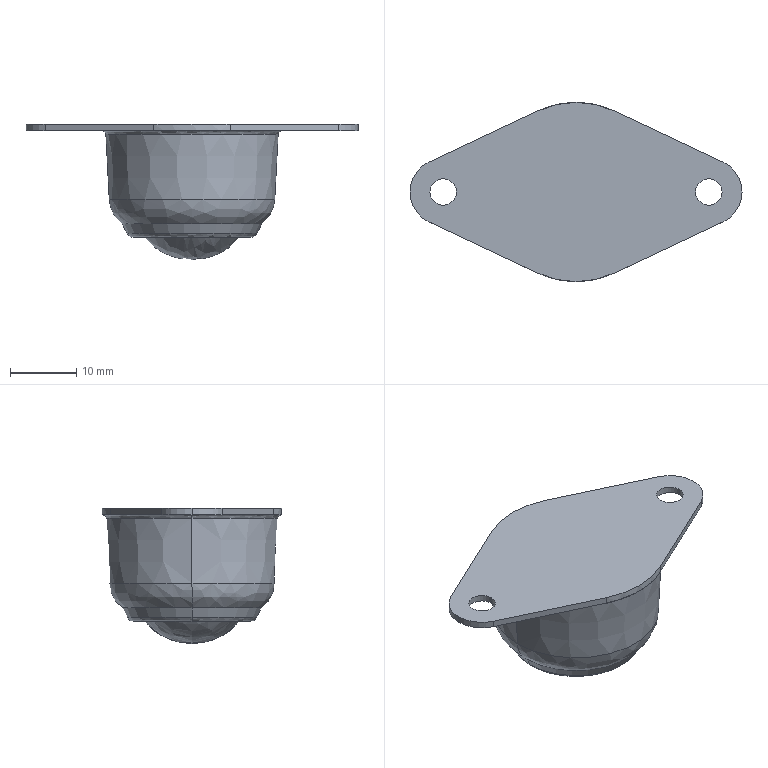Part | SolidWorks | features BaseBody 2 | 2 solids | 32 faces | box 50 x 27 x 20.021 mm | volume 8663 mm3 | cylinder 11 | spline 10 | plane 7 | cone 4 | commonest cylinder face diameters 4 x4 10 x3 15 x2 27 x2
STEP:
#1=CARTESIAN_POINT('',(9.397,0.,-10.));
#2=VERTEX_POINT('',#1);
#3=CARTESIAN_POINT('',(-9.397,0.,-10.));
#4=VERTEX_POINT('',#3);
#5=CARTESIAN_POINT('',(0.,0.,-10.));
#6=DIRECTION('',(0.,0.,-1.));
#7=DIRECTION('',(1.,0.,0.));
#8=AXIS2_PLACEMENT_3D('',#5,#6,#7);
#9=CIRCLE('',#8,9.397);
#10=EDGE_CURVE('',#2,#4,#9,.T.);
#11=ORIENTED_EDGE('',*,*,#10,.F.);
#12=CARTESIAN_POINT('',(0.,0.,-10.));
#13=DIRECTION('',(0.,0.,1.));
#14=DIRECTION('',(1.,0.,0.));
#15=AXIS2_PLACEMENT_3D('',#12,#13,#14);
#16=CIRCLE('',#15,9.397);
#17=EDGE_CURVE('',#2,#4,#16,.T.);
#18=ORIENTED_EDGE('',*,*,#17,.T.);
#19=EDGE_LOOP('',(#11,#18));
#20=FACE_OUTER_BOUND('',#19,.T.);
#21=CARTESIAN_POINT('',(9.397,0.,-10.));
#22=CARTESIAN_POINT('',(9.397,0.,-10.));
#23=CARTESIAN_POINT('',(9.397,0.,-10.));
#24=CARTESIAN_POINT('',(9.397,0.,-10.));
#25=CARTESIAN_POINT('',(9.397,18.793,-10.));
#26=CARTESIAN_POINT('',(9.397,18.793,27.586));
#27=CARTESIAN_POINT('',(9.397,-18.793,27.586));
#28=CARTESIAN_POINT('',(9.397,-18.793,-10.));
#29=CARTESIAN_POINT('',(-9.397,18.793,-10.));
#30=CARTESIAN_POINT('',(-9.397,18.793,27.586));
#31=CARTESIAN_POINT('',(-9.397,-18.793,27.586));
#32=CARTESIAN_POINT('',(-9.397,-18.793,-10.));
#33=CARTESIAN_POINT('',(-9.397,0.,-10.));
#34=CARTESIAN_POINT('',(-9.397,0.,-10.));
#35=CARTESIAN_POINT('',(-9.397,0.,-10.));
#36=CARTESIAN_POINT('',(-9.397,0.,-10.));
#37=(BOUNDED_SURFACE()B_SPLINE_SURFACE(3,3,((#21,#22,#23,#24),(#25,#26,#27,#28),(#29,#30,#31,#32),(#33,#34,#35,#36)),.UNSPECIFIED.,.F.,.F.,.T.)B_SPLINE_SURFACE_WITH_KNOTS((4,4),(4,4),(0.,1.),(0.,1.),.UNSPECIFIED.)GEOMETRIC_REPRESENTATION_ITEM()RATIONAL_B_SPLINE_SURFACE(((1.,0.3333,0.3333,1.),(0.3333,0.1111,0.1111,0.3333),(0.3333,0.1111,0.1111,0.3333),(1.,0.3333,0.3333,1.)))REPRESENTATION_ITEM('')SURFACE());
#38=ADVANCED_FACE('',(#20),#37,.T.);
#39=ORIENTED_EDGE('',*,*,#17,.F.);
#40=ORIENTED_EDGE('',*,*,#10,.T.);
#41=EDGE_LOOP('',(#39,#40));
#42=FACE_OUTER_BOUND('',#41,.T.);
#43=CARTESIAN_POINT('',(9.397,0.,-10.));
#44=CARTESIAN_POINT('',(9.397,0.,-10.));
#45=CARTESIAN_POINT('',(9.397,0.,-10.));
#46=CARTESIAN_POINT('',(9.397,0.,-10.));
#47=CARTESIAN_POINT('',(9.397,-18.793,-10.));
#48=CARTESIAN_POINT('',(9.397,-18.793,-47.586));
#49=CARTESIAN_POINT('',(9.397,18.793,-47.586));
#50=CARTESIAN_POINT('',(9.397,18.793,-10.));
#51=CARTESIAN_POINT('',(-9.397,-18.793,-10.));
#52=CARTESIAN_POINT('',(-9.397,-18.793,-47.586));
#53=CARTESIAN_POINT('',(-9.397,18.793,-47.586));
#54=CARTESIAN_POINT('',(-9.397,18.793,-10.));
#55=CARTESIAN_POINT('',(-9.397,0.,-10.));
#56=CARTESIAN_POINT('',(-9.397,0.,-10.));
#57=CARTESIAN_POINT('',(-9.397,0.,-10.));
#58=CARTESIAN_POINT('',(-9.397,0.,-10.));
#59=(BOUNDED_SURFACE()B_SPLINE_SURFACE(3,3,((#43,#44,#45,#46),(#47,#48,#49,#50),(#51,#52,#53,#54),(#55,#56,#57,#58)),.UNSPECIFIED.,.F.,.F.,.T.)B_SPLINE_SURFACE_WITH_KNOTS((4,4),(4,4),(0.,1.),(0.,1.),.UNSPECIFIED.)GEOMETRIC_REPRESENTATION_ITEM()RATIONAL_B_SPLINE_SURFACE(((1.,0.3333,0.3333,1.),(0.3333,0.1111,0.1111,0.3333),(0.3333,0.1111,0.1111,0.3333),(1.,0.3333,0.3333,1.)))REPRESENTATION_ITEM('')SURFACE());
#60=ADVANCED_FACE('',(#42),#59,.T.);
#61=CLOSED_SHELL('',(#38,#60));
#62=MANIFOLD_SOLID_BREP('',#61);
#63=CARTESIAN_POINT('',(-12.975,0.,-0.4738));
#64=VERTEX_POINT('',#63);
#65=CARTESIAN_POINT('',(12.975,0.,-0.4738));
#66=VERTEX_POINT('',#65);
#67=CARTESIAN_POINT('',(0.,0.,-0.4738));
#68=DIRECTION('',(0.,0.,-1.));
#69=DIRECTION('',(1.,0.,0.));
#70=AXIS2_PLACEMENT_3D('',#67,#68,#69);
#71=CIRCLE('',#70,12.975);
#72=EDGE_CURVE('',#64,#66,#71,.T.);
#73=ORIENTED_EDGE('',*,*,#72,.F.);
#74=CARTESIAN_POINT('',(-13.474,0.,0.));
#75=VERTEX_POINT('',#74);
#76=CARTESIAN_POINT('',(-13.474,0.,-0.5));
#77=DIRECTION('',(0.,-1.,0.));
#78=DIRECTION('',(-1.,0.,0.));
#79=AXIS2_PLACEMENT_3D('',#76,#77,#78);
#80=CIRCLE('',#79,0.5);
#81=EDGE_CURVE('',#64,#75,#80,.T.);
#82=ORIENTED_EDGE('',*,*,#81,.T.);
#83=CARTESIAN_POINT('',(13.474,0.,0.));
#84=VERTEX_POINT('',#83);
#85=CARTESIAN_POINT('',(-13.474,0.,0.));
#86=CARTESIAN_POINT('',(-13.474,26.949,0.));
#87=CARTESIAN_POINT('',(13.474,26.949,0.));
#88=CARTESIAN_POINT('',(13.474,0.,0.));
#89=(BOUNDED_CURVE()B_SPLINE_CURVE(3,(#85,#86,#87,#88),.UNSPECIFIED.,.F.,.F.)B_SPLINE_CURVE_WITH_KNOTS((4,4),(0.,1.),.UNSPECIFIED.)CURVE()GEOMETRIC_REPRESENTATION_ITEM()RATIONAL_B_SPLINE_CURVE((1.,0.3333,0.3333,1.))REPRESENTATION_ITEM(''));
#90=EDGE_CURVE('',#75,#84,#89,.T.);
#91=ORIENTED_EDGE('',*,*,#90,.T.);
#92=CARTESIAN_POINT('',(13.474,0.,-0.5));
#93=DIRECTION('',(0.,1.,0.));
#94=DIRECTION('',(1.,0.,0.));
#95=AXIS2_PLACEMENT_3D('',#92,#93,#94);
#96=CIRCLE('',#95,0.5);
#97=EDGE_CURVE('',#66,#84,#96,.T.);
#98=ORIENTED_EDGE('',*,*,#97,.F.);
#99=EDGE_LOOP('',(#73,#82,#91,#98));
#100=FACE_OUTER_BOUND('',#99,.T.);
#101=CARTESIAN_POINT('',(12.975,0.,-0.4738));
#102=CARTESIAN_POINT('',(12.975,25.95,-0.4738));
#103=CARTESIAN_POINT('',(-12.975,25.95,-0.4738));
#104=CARTESIAN_POINT('',(-12.975,0.,-0.4738));
#105=CARTESIAN_POINT('',(12.99,0.,-0.1933));
#106=CARTESIAN_POINT('',(12.99,25.98,-0.1933));
#107=CARTESIAN_POINT('',(-12.99,25.98,-0.1933));
#108=CARTESIAN_POINT('',(-12.99,0.,-0.1933));
#109=CARTESIAN_POINT('',(13.194,0.,0.));
#110=CARTESIAN_POINT('',(13.194,26.387,0.));
#111=CARTESIAN_POINT('',(-13.194,26.387,0.));
#112=CARTESIAN_POINT('',(-13.194,0.,0.));
#113=CARTESIAN_POINT('',(13.474,0.,0.));
#114=CARTESIAN_POINT('',(13.474,26.949,0.));
#115=CARTESIAN_POINT('',(-13.474,26.949,0.));
#116=CARTESIAN_POINT('',(-13.474,0.,0.));
#117=(BOUNDED_SURFACE()B_SPLINE_SURFACE(3,3,((#101,#102,#103,#104),(#105,#106,#107,#108),(#109,#110,#111,#112),(#113,#114,#115,#116)),.UNSPECIFIED.,.F.,.F.,.T.)B_SPLINE_SURFACE_WITH_KNOTS((4,4),(4,4),(0.,1.),(0.,1.),.UNSPECIFIED.)GEOMETRIC_REPRESENTATION_ITEM()RATIONAL_B_SPLINE_SURFACE(((1.,0.3333,0.3333,1.),(0.8169,0.2723,0.2723,0.8169),(0.8169,0.2723,0.2723,0.8169),(1.,0.3333,0.3333,1.)))REPRESENTATION_ITEM('')SURFACE());
#118=ADVANCED_FACE('',(#100),#117,.F.);
#119=CARTESIAN_POINT('',(-10.5,0.,-14.));
#120=VERTEX_POINT('',#119);
#121=CARTESIAN_POINT('',(10.5,0.,-14.));
#122=VERTEX_POINT('',#121);
#123=CARTESIAN_POINT('',(0.,0.,-14.));
#124=DIRECTION('',(0.,0.,1.));
#125=DIRECTION('',(-1.,0.,0.));
#126=AXIS2_PLACEMENT_3D('',#123,#124,#125);
#127=CIRCLE('',#126,10.5);
#128=EDGE_CURVE('',#120,#122,#127,.T.);
#129=ORIENTED_EDGE('',*,*,#128,.T.);
#130=CARTESIAN_POINT('',(12.461,0.,-10.286));
#131=VERTEX_POINT('',#130);
#132=CARTESIAN_POINT('',(7.468,0.,-10.024));
#133=DIRECTION('',(0.,-1.,0.));
#134=DIRECTION('',(1.,0.,0.));
#135=AXIS2_PLACEMENT_3D('',#132,#133,#134);
#136=CIRCLE('',#135,5.);
#137=EDGE_CURVE('',#122,#131,#136,.T.);
#138=ORIENTED_EDGE('',*,*,#137,.T.);
#139=CARTESIAN_POINT('',(-12.461,0.,-10.286));
#140=VERTEX_POINT('',#139);
#141=CARTESIAN_POINT('',(0.,0.,-10.286));
#142=DIRECTION('',(0.,0.,1.));
#143=DIRECTION('',(1.,0.,0.));
#144=AXIS2_PLACEMENT_3D('',#141,#142,#143);
#145=CIRCLE('',#144,12.461);
#146=EDGE_CURVE('',#140,#131,#145,.T.);
#147=ORIENTED_EDGE('',*,*,#146,.F.);
#148=CARTESIAN_POINT('',(-7.468,0.,-10.024));
#149=DIRECTION('',(0.,1.,0.));
#150=DIRECTION('',(-1.,0.,0.));
#151=AXIS2_PLACEMENT_3D('',#148,#149,#150);
#152=CIRCLE('',#151,5.);
#153=EDGE_CURVE('',#120,#140,#152,.T.);
#154=ORIENTED_EDGE('',*,*,#153,.F.);
#155=EDGE_LOOP('',(#129,#138,#147,#154));
#156=FACE_OUTER_BOUND('',#155,.T.);
#157=CARTESIAN_POINT('',(10.5,0.,-14.));
#158=CARTESIAN_POINT('',(10.5,-21.,-14.));
#159=CARTESIAN_POINT('',(-10.5,-21.,-14.));
#160=CARTESIAN_POINT('',(-10.5,0.,-14.));
#161=CARTESIAN_POINT('',(11.686,0.,-13.095));
#162=CARTESIAN_POINT('',(11.686,-23.373,-13.095));
#163=CARTESIAN_POINT('',(-11.686,-23.373,-13.095));
#164=CARTESIAN_POINT('',(-11.686,0.,-13.095));
#165=CARTESIAN_POINT('',(12.383,0.,-11.776));
#166=CARTESIAN_POINT('',(12.383,-24.766,-11.776));
#167=CARTESIAN_POINT('',(-12.383,-24.766,-11.776));
#168=CARTESIAN_POINT('',(-12.383,0.,-11.776));
#169=CARTESIAN_POINT('',(12.461,0.,-10.286));
#170=CARTESIAN_POINT('',(12.461,-24.922,-10.286));
#171=CARTESIAN_POINT('',(-12.461,-24.922,-10.286));
#172=CARTESIAN_POINT('',(-12.461,0.,-10.286));
#173=(BOUNDED_SURFACE()B_SPLINE_SURFACE(3,3,((#157,#158,#159,#160),(#161,#162,#163,#164),(#165,#166,#167,#168),(#169,#170,#171,#172)),.UNSPECIFIED.,.F.,.F.,.T.)B_SPLINE_SURFACE_WITH_KNOTS((4,4),(4,4),(0.,1.),(0.,1.),.UNSPECIFIED.)GEOMETRIC_REPRESENTATION_ITEM()RATIONAL_B_SPLINE_SURFACE(((1.,0.3333,0.3333,1.),(0.9384,0.3128,0.3128,0.9384),(0.9384,0.3128,0.3128,0.9384),(1.,0.3333,0.3333,1.)))REPRESENTATION_ITEM('')SURFACE());
#174=ADVANCED_FACE('',(#156),#173,.T.);
#175=CARTESIAN_POINT('',(-8.882,0.,-16.));
#176=VERTEX_POINT('',#175);
#177=CARTESIAN_POINT('',(8.882,0.,-16.));
#178=VERTEX_POINT('',#177);
#179=CARTESIAN_POINT('',(-8.882,0.,-16.));
#180=CARTESIAN_POINT('',(-8.882,-17.764,-16.));
#181=CARTESIAN_POINT('',(8.882,-17.764,-16.));
#182=CARTESIAN_POINT('',(8.882,0.,-16.));
#183=(BOUNDED_CURVE()B_SPLINE_CURVE(3,(#179,#180,#181,#182),.UNSPECIFIED.,.F.,.F.)B_SPLINE_CURVE_WITH_KNOTS((4,4),(0.,1.),.UNSPECIFIED.)CURVE()GEOMETRIC_REPRESENTATION_ITEM()RATIONAL_B_SPLINE_CURVE((1.,0.3333,0.3333,1.))REPRESENTATION_ITEM(''));
#184=EDGE_CURVE('',#176,#178,#183,.T.);
#185=ORIENTED_EDGE('',*,*,#184,.T.);
#186=CARTESIAN_POINT('',(9.776,0.,-15.447));
#187=VERTEX_POINT('',#186);
#188=CARTESIAN_POINT('',(8.882,0.,-15.));
#189=DIRECTION('',(0.,-1.,0.));
#190=DIRECTION('',(1.,0.,0.));
#191=AXIS2_PLACEMENT_3D('',#188,#189,#190);
#192=CIRCLE('',#191,1.);
#193=EDGE_CURVE('',#178,#187,#192,.T.);
#194=ORIENTED_EDGE('',*,*,#193,.T.);
#195=CARTESIAN_POINT('',(-9.776,0.,-15.447));
#196=VERTEX_POINT('',#195);
#197=CARTESIAN_POINT('',(0.,0.,-15.447));
#198=DIRECTION('',(0.,0.,1.));
#199=DIRECTION('',(1.,0.,0.));
#200=AXIS2_PLACEMENT_3D('',#197,#198,#199);
#201=CIRCLE('',#200,9.776);
#202=EDGE_CURVE('',#196,#187,#201,.T.);
#203=ORIENTED_EDGE('',*,*,#202,.F.);
#204=CARTESIAN_POINT('',(-8.882,0.,-15.));
#205=DIRECTION('',(0.,1.,0.));
#206=DIRECTION('',(-1.,0.,0.));
#207=AXIS2_PLACEMENT_3D('',#204,#205,#206);
#208=CIRCLE('',#207,1.);
#209=EDGE_CURVE('',#176,#196,#208,.T.);
#210=ORIENTED_EDGE('',*,*,#209,.F.);
#211=EDGE_LOOP('',(#185,#194,#203,#210));
#212=FACE_OUTER_BOUND('',#211,.T.);
#213=CARTESIAN_POINT('',(8.882,0.,-16.));
#214=CARTESIAN_POINT('',(8.882,-17.764,-16.));
#215=CARTESIAN_POINT('',(-8.882,-17.764,-16.));
#216=CARTESIAN_POINT('',(-8.882,0.,-16.));
#217=CARTESIAN_POINT('',(9.271,0.,-16.));
#218=CARTESIAN_POINT('',(9.271,-18.542,-16.));
#219=CARTESIAN_POINT('',(-9.271,-18.542,-16.));
#220=CARTESIAN_POINT('',(-9.271,0.,-16.));
#221=CARTESIAN_POINT('',(9.602,0.,-15.795));
#222=CARTESIAN_POINT('',(9.602,-19.205,-15.795));
#223=CARTESIAN_POINT('',(-9.602,-19.205,-15.795));
#224=CARTESIAN_POINT('',(-9.602,0.,-15.795));
#225=CARTESIAN_POINT('',(9.776,0.,-15.447));
#226=CARTESIAN_POINT('',(9.776,-19.553,-15.447));
#227=CARTESIAN_POINT('',(-9.776,-19.553,-15.447));
#228=CARTESIAN_POINT('',(-9.776,0.,-15.447));
#229=(BOUNDED_SURFACE()B_SPLINE_SURFACE(3,3,((#213,#214,#215,#216),(#217,#218,#219,#220),(#221,#222,#223,#224),(#225,#226,#227,#228)),.UNSPECIFIED.,.F.,.F.,.T.)B_SPLINE_SURFACE_WITH_KNOTS((4,4),(4,4),(0.,1.),(0.,1.),.UNSPECIFIED.)GEOMETRIC_REPRESENTATION_ITEM()RATIONAL_B_SPLINE_SURFACE(((1.,0.3333,0.3333,1.),(0.9004,0.3001,0.3001,0.9004),(0.9004,0.3001,0.3001,0.9004),(1.,0.3333,0.3333,1.)))REPRESENTATION_ITEM('')SURFACE());
#230=ADVANCED_FACE('',(#212),#229,.T.);
#231=CARTESIAN_POINT('',(7.5,0.,-15.661));
#232=VERTEX_POINT('',#231);
#233=CARTESIAN_POINT('',(-7.5,0.,-15.661));
#234=VERTEX_POINT('',#233);
#235=CARTESIAN_POINT('',(0.,0.,-15.661));
#236=DIRECTION('',(0.,0.,-1.));
#237=DIRECTION('',(1.,0.,0.));
#238=AXIS2_PLACEMENT_3D('',#235,#236,#237);
#239=CIRCLE('',#238,7.5);
#240=EDGE_CURVE('',#232,#234,#239,.T.);
#241=ORIENTED_EDGE('',*,*,#240,.T.);
#242=CARTESIAN_POINT('',(0.,0.,-15.661));
#243=DIRECTION('',(0.,0.,-1.));
#244=DIRECTION('',(1.,0.,0.));
#245=AXIS2_PLACEMENT_3D('',#242,#243,#244);
#246=CIRCLE('',#245,7.5);
#247=EDGE_CURVE('',#234,#232,#246,.T.);
#248=ORIENTED_EDGE('',*,*,#247,.T.);
#249=EDGE_LOOP('',(#241,#248));
#250=FACE_BOUND('',#249,.T.);
#251=CARTESIAN_POINT('',(9.397,0.,-10.));
#252=VERTEX_POINT('',#251);
#253=CARTESIAN_POINT('',(-9.397,0.,-10.));
#254=VERTEX_POINT('',#253);
#255=CARTESIAN_POINT('',(0.,0.,-10.));
#256=DIRECTION('',(0.,0.,-1.));
#257=DIRECTION('',(1.,0.,0.));
#258=AXIS2_PLACEMENT_3D('',#255,#256,#257);
#259=CIRCLE('',#258,9.397);
#260=EDGE_CURVE('',#252,#254,#259,.T.);
#261=ORIENTED_EDGE('',*,*,#260,.F.);
#262=CARTESIAN_POINT('',(0.,0.,-10.));
#263=DIRECTION('',(0.,0.,1.));
#264=DIRECTION('',(1.,0.,0.));
#265=AXIS2_PLACEMENT_3D('',#262,#263,#264);
#266=CIRCLE('',#265,9.397);
#267=EDGE_CURVE('',#252,#254,#266,.T.);
#268=ORIENTED_EDGE('',*,*,#267,.T.);
#269=EDGE_LOOP('',(#261,#268));
#270=FACE_OUTER_BOUND('',#269,.T.);
#271=CARTESIAN_POINT('',(9.397,0.,-10.));
#272=CARTESIAN_POINT('',(9.397,0.,-10.));
#273=CARTESIAN_POINT('',(9.397,0.,-10.));
#274=CARTESIAN_POINT('',(9.397,0.,-10.));
#275=CARTESIAN_POINT('',(9.397,-18.793,-10.));
#276=CARTESIAN_POINT('',(9.397,-18.793,-47.586));
#277=CARTESIAN_POINT('',(9.397,18.793,-47.586));
#278=CARTESIAN_POINT('',(9.397,18.793,-10.));
#279=CARTESIAN_POINT('',(-9.397,-18.793,-10.));
#280=CARTESIAN_POINT('',(-9.397,-18.793,-47.586));
#281=CARTESIAN_POINT('',(-9.397,18.793,-47.586));
#282=CARTESIAN_POINT('',(-9.397,18.793,-10.));
#283=CARTESIAN_POINT('',(-9.397,0.,-10.));
#284=CARTESIAN_POINT('',(-9.397,0.,-10.));
#285=CARTESIAN_POINT('',(-9.397,0.,-10.));
#286=CARTESIAN_POINT('',(-9.397,0.,-10.));
#287=(BOUNDED_SURFACE()B_SPLINE_SURFACE(3,3,((#271,#272,#273,#274),(#275,#276,#277,#278),(#279,#280,#281,#282),(#283,#284,#285,#286)),.UNSPECIFIED.,.F.,.F.,.T.)B_SPLINE_SURFACE_WITH_KNOTS((4,4),(4,4),(0.,1.),(0.,1.),.UNSPECIFIED.)GEOMETRIC_REPRESENTATION_ITEM()RATIONAL_B_SPLINE_SURFACE(((1.,0.3333,0.3333,1.),(0.3333,0.1111,0.1111,0.3333),(0.3333,0.1111,0.1111,0.3333),(1.,0.3333,0.3333,1.)))REPRESENTATION_ITEM('')SURFACE());
#288=ADVANCED_FACE('',(#250,#270),#287,.F.);
#289=CARTESIAN_POINT('',(-25.,0.,1.));
#290=VERTEX_POINT('',#289);
#291=CARTESIAN_POINT('',(-22.125,-4.526,1.));
#292=VERTEX_POINT('',#291);
#293=CARTESIAN_POINT('',(-20.,0.,1.));
#294=DIRECTION('',(0.,0.,1.));
#295=DIRECTION('',(-1.,0.,0.));
#296=AXIS2_PLACEMENT_3D('',#293,#294,#295);
#297=CIRCLE('',#296,5.);
#298=EDGE_CURVE('',#290,#292,#297,.T.);
#299=ORIENTED_EDGE('',*,*,#298,.F.);
#300=CARTESIAN_POINT('',(-25.,0.,0.));
#301=VERTEX_POINT('',#300);
#302=CARTESIAN_POINT('',(-25.,0.,1.));
#303=DIRECTION('',(0.,0.,-1.));
#304=VECTOR('',#303,1000.);
#305=LINE('',#302,#304);
#306=EDGE_CURVE('',#290,#301,#305,.T.);
#307=ORIENTED_EDGE('',*,*,#306,.T.);
#308=CARTESIAN_POINT('',(-22.125,-4.526,0.));
#309=VERTEX_POINT('',#308);
#310=CARTESIAN_POINT('',(-20.,0.,0.));
#311=DIRECTION('',(0.,0.,1.));
#312=DIRECTION('',(-1.,0.,0.));
#313=AXIS2_PLACEMENT_3D('',#310,#311,#312);
#314=CIRCLE('',#313,5.);
#315=EDGE_CURVE('',#301,#309,#314,.T.);
#316=ORIENTED_EDGE('',*,*,#315,.T.);
#317=CARTESIAN_POINT('',(-22.125,-4.526,1.));
#318=DIRECTION('',(0.,0.,1.));
#319=VECTOR('',#318,1000.);
#320=LINE('',#317,#319);
#321=EDGE_CURVE('',#309,#292,#320,.T.);
#322=ORIENTED_EDGE('',*,*,#321,.T.);
#323=EDGE_LOOP('',(#299,#307,#316,#322));
#324=FACE_OUTER_BOUND('',#323,.T.);
#325=CARTESIAN_POINT('',(-20.,0.,1.));
#326=DIRECTION('',(0.,0.,-1.));
#327=DIRECTION('',(-1.,0.,0.));
#328=AXIS2_PLACEMENT_3D('',#325,#326,#327);
#329=CYLINDRICAL_SURFACE('',#328,5.);
#330=ADVANCED_FACE('',(#324),#329,.T.);
#331=CARTESIAN_POINT('',(22.,0.,1.));
#332=VERTEX_POINT('',#331);
#333=CARTESIAN_POINT('',(18.,0.,1.));
#334=VERTEX_POINT('',#333);
#335=CARTESIAN_POINT('',(20.,0.,1.));
#336=DIRECTION('',(0.,0.,-1.));
#337=DIRECTION('',(-1.,0.,0.));
#338=AXIS2_PLACEMENT_3D('',#335,#336,#337);
#339=CIRCLE('',#338,2.);
#340=EDGE_CURVE('',#332,#334,#339,.T.);
#341=ORIENTED_EDGE('',*,*,#340,.F.);
#342=CARTESIAN_POINT('',(22.,0.,0.));
#343=VERTEX_POINT('',#342);
#344=CARTESIAN_POINT('',(22.,0.,1.));
#345=DIRECTION('',(0.,0.,-1.));
#346=VECTOR('',#345,1000.);
#347=LINE('',#344,#346);
#348=EDGE_CURVE('',#332,#343,#347,.T.);
#349=ORIENTED_EDGE('',*,*,#348,.T.);
#350=CARTESIAN_POINT('',(18.,0.,0.));
#351=VERTEX_POINT('',#350);
#352=CARTESIAN_POINT('',(20.,0.,0.));
#353=DIRECTION('',(0.,0.,1.));
#354=DIRECTION('',(-1.,0.,0.));
#355=AXIS2_PLACEMENT_3D('',#352,#353,#354);
#356=CIRCLE('',#355,2.);
#357=EDGE_CURVE('',#351,#343,#356,.T.);
#358=ORIENTED_EDGE('',*,*,#357,.F.);
#359=CARTESIAN_POINT('',(18.,0.,1.));
#360=DIRECTION('',(0.,0.,-1.));
#361=VECTOR('',#360,1000.);
#362=LINE('',#359,#361);
#363=EDGE_CURVE('',#334,#351,#362,.T.);
#364=ORIENTED_EDGE('',*,*,#363,.F.);
#365=EDGE_LOOP('',(#341,#349,#358,#364));
#366=FACE_OUTER_BOUND('',#365,.T.);
#367=CARTESIAN_POINT('',(20.,0.,1.));
#368=DIRECTION('',(0.,0.,-1.));
#369=DIRECTION('',(-1.,0.,0.));
#370=AXIS2_PLACEMENT_3D('',#367,#368,#369);
#371=CYLINDRICAL_SURFACE('',#370,2.);
#372=ADVANCED_FACE('',(#366),#371,.F.);
#373=CARTESIAN_POINT('',(-18.,0.,1.));
#374=VERTEX_POINT('',#373);
#375=CARTESIAN_POINT('',(-22.,0.,1.));
#376=VERTEX_POINT('',#375);
#377=CARTESIAN_POINT('',(-20.,0.,1.));
#378=DIRECTION('',(0.,0.,-1.));
#379=DIRECTION('',(-1.,0.,0.));
#380=AXIS2_PLACEMENT_3D('',#377,#378,#379);
#381=CIRCLE('',#380,2.);
#382=EDGE_CURVE('',#374,#376,#381,.T.);
#383=ORIENTED_EDGE('',*,*,#382,.F.);
#384=CARTESIAN_POINT('',(-18.,0.,0.));
#385=VERTEX_POINT('',#384);
#386=CARTESIAN_POINT('',(-18.,0.,1.));
#387=DIRECTION('',(0.,0.,-1.));
#388=VECTOR('',#387,1000.);
#389=LINE('',#386,#388);
#390=EDGE_CURVE('',#374,#385,#389,.T.);
#391=ORIENTED_EDGE('',*,*,#390,.T.);
#392=CARTESIAN_POINT('',(-22.,0.,0.));
#393=VERTEX_POINT('',#392);
#394=CARTESIAN_POINT('',(-20.,0.,0.));
#395=DIRECTION('',(0.,0.,1.));
#396=DIRECTION('',(-1.,0.,0.));
#397=AXIS2_PLACEMENT_3D('',#394,#395,#396);
#398=CIRCLE('',#397,2.);
#399=EDGE_CURVE('',#393,#385,#398,.T.);
#400=ORIENTED_EDGE('',*,*,#399,.F.);
#401=CARTESIAN_POINT('',(-22.,0.,1.));
#402=DIRECTION('',(0.,0.,-1.));
#403=VECTOR('',#402,1000.);
#404=LINE('',#401,#403);
#405=EDGE_CURVE('',#376,#393,#404,.T.);
#406=ORIENTED_EDGE('',*,*,#405,.F.);
#407=EDGE_LOOP('',(#383,#391,#400,#406));
#408=FACE_OUTER_BOUND('',#407,.T.);
#409=CARTESIAN_POINT('',(-20.,0.,1.));
#410=DIRECTION('',(0.,0.,-1.));
#411=DIRECTION('',(-1.,0.,0.));
#412=AXIS2_PLACEMENT_3D('',#409,#410,#411);
#413=CYLINDRICAL_SURFACE('',#412,2.);
#414=ADVANCED_FACE('',(#408),#413,.F.);
#415=CARTESIAN_POINT('',(0.,0.,-10.286));
#416=DIRECTION('',(0.,0.,1.));
#417=DIRECTION('',(1.,0.,0.));
#418=AXIS2_PLACEMENT_3D('',#415,#416,#417);
#419=CIRCLE('',#418,12.461);
#420=EDGE_CURVE('',#131,#140,#419,.T.);
#421=ORIENTED_EDGE('',*,*,#420,.T.);
#422=CARTESIAN_POINT('',(-12.975,0.,-0.4738));
#423=DIRECTION('',(-0.05234,0.,0.9986));
#424=VECTOR('',#423,1000.);
#425=LINE('',#422,#424);
#426=EDGE_CURVE('',#140,#64,#425,.T.);
#427=ORIENTED_EDGE('',*,*,#426,.T.);
#428=ORIENTED_EDGE('',*,*,#72,.T.);
#429=CARTESIAN_POINT('',(12.975,0.,-0.4738));
#430=DIRECTION('',(0.05234,0.,0.9986));
#431=VECTOR('',#430,1000.);
#432=LINE('',#429,#431);
#433=EDGE_CURVE('',#131,#66,#432,.T.);
#434=ORIENTED_EDGE('',*,*,#433,.F.);
#435=EDGE_LOOP('',(#421,#427,#428,#434));
#436=FACE_OUTER_BOUND('',#435,.T.);
#437=CARTESIAN_POINT('',(0.,0.,-0.4738));
#438=DIRECTION('',(0.,0.,1.));
#439=DIRECTION('',(1.,0.,0.));
#440=AXIS2_PLACEMENT_3D('',#437,#438,#439);
#441=CONICAL_SURFACE('',#440,12.975,0.05236);
#442=ADVANCED_FACE('',(#436),#441,.T.);
#443=CARTESIAN_POINT('',(0.,0.,-15.447));
#444=DIRECTION('',(0.,0.,1.));
#445=DIRECTION('',(1.,0.,0.));
#446=AXIS2_PLACEMENT_3D('',#443,#444,#445);
#447=CIRCLE('',#446,9.776);
#448=EDGE_CURVE('',#187,#196,#447,.T.);
#449=ORIENTED_EDGE('',*,*,#448,.T.);
#450=CARTESIAN_POINT('',(-10.5,0.,-14.));
#451=DIRECTION('',(-0.4472,0.,0.8944));
#452=VECTOR('',#451,1000.);
#453=LINE('',#450,#452);
#454=EDGE_CURVE('',#196,#120,#453,.T.);
#455=ORIENTED_EDGE('',*,*,#454,.T.);
#456=CARTESIAN_POINT('',(0.,0.,-14.));
#457=DIRECTION('',(0.,0.,1.));
#458=DIRECTION('',(-1.,0.,0.));
#459=AXIS2_PLACEMENT_3D('',#456,#457,#458);
#460=CIRCLE('',#459,10.5);
#461=EDGE_CURVE('',#122,#120,#460,.T.);
#462=ORIENTED_EDGE('',*,*,#461,.F.);
#463=CARTESIAN_POINT('',(10.5,0.,-14.));
#464=DIRECTION('',(0.4472,0.,0.8944));
#465=VECTOR('',#464,1000.);
#466=LINE('',#463,#465);
#467=EDGE_CURVE('',#187,#122,#466,.T.);
#468=ORIENTED_EDGE('',*,*,#467,.F.);
#469=EDGE_LOOP('',(#449,#455,#462,#468));
#470=FACE_OUTER_BOUND('',#469,.T.);
#471=CARTESIAN_POINT('',(0.,0.,-14.));
#472=DIRECTION('',(0.,0.,1.));
#473=DIRECTION('',(1.,0.,0.));
#474=AXIS2_PLACEMENT_3D('',#471,#472,#473);
#475=CONICAL_SURFACE('',#474,10.5,0.4636);
#476=ADVANCED_FACE('',(#470),#475,.T.);
#477=CARTESIAN_POINT('',(-7.5,0.,-16.));
#478=VERTEX_POINT('',#477);
#479=CARTESIAN_POINT('',(7.5,0.,-16.));
#480=VERTEX_POINT('',#479);
#481=CARTESIAN_POINT('',(0.,0.,-16.));
#482=DIRECTION('',(0.,0.,1.));
#483=DIRECTION('',(1.,0.,0.));
#484=AXIS2_PLACEMENT_3D('',#481,#482,#483);
#485=CIRCLE('',#484,7.5);
#486=EDGE_CURVE('',#478,#480,#485,.T.);
#487=ORIENTED_EDGE('',*,*,#486,.F.);
#488=CARTESIAN_POINT('',(-7.5,0.,-16.));
#489=DIRECTION('',(0.,0.,1.));
#490=VECTOR('',#489,1000.);
#491=LINE('',#488,#490);
#492=EDGE_CURVE('',#478,#234,#491,.T.);
#493=ORIENTED_EDGE('',*,*,#492,.T.);
#494=ORIENTED_EDGE('',*,*,#240,.F.);
#495=CARTESIAN_POINT('',(7.5,0.,-16.));
#496=DIRECTION('',(0.,0.,1.));
#497=VECTOR('',#496,1000.);
#498=LINE('',#495,#497);
#499=EDGE_CURVE('',#480,#232,#498,.T.);
#500=ORIENTED_EDGE('',*,*,#499,.F.);
#501=EDGE_LOOP('',(#487,#493,#494,#500));
#502=FACE_OUTER_BOUND('',#501,.T.);
#503=CARTESIAN_POINT('',(0.,0.,-16.));
#504=DIRECTION('',(0.,0.,1.));
#505=DIRECTION('',(1.,0.,0.));
#506=AXIS2_PLACEMENT_3D('',#503,#504,#505);
#507=CYLINDRICAL_SURFACE('',#506,7.5);
#508=ADVANCED_FACE('',(#502),#507,.F.);
#509=CARTESIAN_POINT('',(5.738,12.22,1.));
#510=VERTEX_POINT('',#509);
#511=CARTESIAN_POINT('',(-5.738,12.22,1.));
#512=VERTEX_POINT('',#511);
#513=CARTESIAN_POINT('',(0.,0.,1.));
#514=DIRECTION('',(0.,0.,1.));
#515=DIRECTION('',(-1.,0.,0.));
#516=AXIS2_PLACEMENT_3D('',#513,#514,#515);
#517=CIRCLE('',#516,13.5);
#518=EDGE_CURVE('',#510,#512,#517,.T.);
#519=ORIENTED_EDGE('',*,*,#518,.T.);
#520=CARTESIAN_POINT('',(-22.125,4.526,1.));
#521=VERTEX_POINT('',#520);
#522=CARTESIAN_POINT('',(-5.738,12.22,1.));
#523=DIRECTION('',(-0.9052,-0.425,0.));
#524=VECTOR('',#523,1000.);
#525=LINE('',#522,#524);
#526=EDGE_CURVE('',#512,#521,#525,.T.);
#527=ORIENTED_EDGE('',*,*,#526,.T.);
#528=CARTESIAN_POINT('',(-20.,0.,1.));
#529=DIRECTION('',(0.,0.,1.));
#530=DIRECTION('',(-1.,0.,0.));
#531=AXIS2_PLACEMENT_3D('',#528,#529,#530);
#532=CIRCLE('',#531,5.);
#533=EDGE_CURVE('',#521,#290,#532,.T.);
#534=ORIENTED_EDGE('',*,*,#533,.T.);
#535=ORIENTED_EDGE('',*,*,#298,.T.);
#536=CARTESIAN_POINT('',(-5.737,-12.22,1.));
#537=VERTEX_POINT('',#536);
#538=CARTESIAN_POINT('',(-22.125,-4.526,1.));
#539=DIRECTION('',(0.9052,-0.425,0.));
#540=VECTOR('',#539,1000.);
#541=LINE('',#538,#540);
#542=EDGE_CURVE('',#292,#537,#541,.T.);
#543=ORIENTED_EDGE('',*,*,#542,.T.);
#544=CARTESIAN_POINT('',(5.738,-12.22,1.));
#545=VERTEX_POINT('',#544);
#546=CARTESIAN_POINT('',(0.,0.,1.));
#547=DIRECTION('',(0.,0.,1.));
#548=DIRECTION('',(-1.,0.,0.));
#549=AXIS2_PLACEMENT_3D('',#546,#547,#548);
#550=CIRCLE('',#549,13.5);
#551=EDGE_CURVE('',#537,#545,#550,.T.);
#552=ORIENTED_EDGE('',*,*,#551,.T.);
#553=CARTESIAN_POINT('',(22.125,-4.526,1.));
#554=VERTEX_POINT('',#553);
#555=CARTESIAN_POINT('',(5.738,-12.22,1.));
#556=DIRECTION('',(0.9052,0.425,0.));
#557=VECTOR('',#556,1000.);
#558=LINE('',#555,#557);
#559=EDGE_CURVE('',#545,#554,#558,.T.);
#560=ORIENTED_EDGE('',*,*,#559,.T.);
#561=CARTESIAN_POINT('',(22.125,4.526,1.));
#562=VERTEX_POINT('',#561);
#563=CARTESIAN_POINT('',(20.,0.,1.));
#564=DIRECTION('',(0.,0.,1.));
#565=DIRECTION('',(-1.,0.,0.));
#566=AXIS2_PLACEMENT_3D('',#563,#564,#565);
#567=CIRCLE('',#566,5.);
#568=EDGE_CURVE('',#554,#562,#567,.T.);
#569=ORIENTED_EDGE('',*,*,#568,.T.);
#570=CARTESIAN_POINT('',(22.125,4.526,1.));
#571=DIRECTION('',(-0.9052,0.425,0.));
#572=VECTOR('',#571,1000.);
#573=LINE('',#570,#572);
#574=EDGE_CURVE('',#562,#510,#573,.T.);
#575=ORIENTED_EDGE('',*,*,#574,.T.);
#576=EDGE_LOOP('',(#519,#527,#534,#535,#543,#552,#560,#569,#575));
#577=FACE_OUTER_BOUND('',#576,.T.);
#578=CARTESIAN_POINT('',(20.,0.,1.));
#579=DIRECTION('',(0.,0.,-1.));
#580=DIRECTION('',(-1.,0.,0.));
#581=AXIS2_PLACEMENT_3D('',#578,#579,#580);
#582=CIRCLE('',#581,2.);
#583=EDGE_CURVE('',#334,#332,#582,.T.);
#584=ORIENTED_EDGE('',*,*,#583,.T.);
#585=ORIENTED_EDGE('',*,*,#340,.T.);
#586=EDGE_LOOP('',(#584,#585));
#587=FACE_BOUND('',#586,.T.);
#588=CARTESIAN_POINT('',(-20.,0.,1.));
#589=DIRECTION('',(0.,0.,-1.));
#590=DIRECTION('',(-1.,0.,0.));
#591=AXIS2_PLACEMENT_3D('',#588,#589,#590);
#592=CIRCLE('',#591,2.);
#593=EDGE_CURVE('',#376,#374,#592,.T.);
#594=ORIENTED_EDGE('',*,*,#593,.T.);
#595=ORIENTED_EDGE('',*,*,#382,.T.);
#596=EDGE_LOOP('',(#594,#595));
#597=FACE_BOUND('',#596,.T.);
#598=CARTESIAN_POINT('',(-20.,0.,1.));
#599=DIRECTION('',(0.,0.,1.));
#600=DIRECTION('',(1.,0.,0.));
#601=AXIS2_PLACEMENT_3D('',#598,#599,#600);
#602=PLANE('',#601);
#603=ADVANCED_FACE('',(#577,#587,#597),#602,.T.);
#604=CARTESIAN_POINT('',(-22.125,4.526,0.));
#605=VERTEX_POINT('',#604);
#606=CARTESIAN_POINT('',(-22.125,4.526,1.));
#607=DIRECTION('',(0.,0.,-1.));
#608=VECTOR('',#607,1000.);
#609=LINE('',#606,#608);
#610=EDGE_CURVE('',#521,#605,#609,.T.);
#611=ORIENTED_EDGE('',*,*,#610,.F.);
#612=ORIENTED_EDGE('',*,*,#526,.F.);
#613=CARTESIAN_POINT('',(-5.738,12.22,0.));
#614=VERTEX_POINT('',#613);
#615=CARTESIAN_POINT('',(-5.738,12.22,1.));
#616=DIRECTION('',(0.,0.,1.));
#617=VECTOR('',#616,1000.);
#618=LINE('',#615,#617);
#619=EDGE_CURVE('',#614,#512,#618,.T.);
#620=ORIENTED_EDGE('',*,*,#619,.F.);
#621=CARTESIAN_POINT('',(-5.738,12.22,0.));
#622=DIRECTION('',(0.9052,0.425,0.));
#623=VECTOR('',#622,1000.);
#624=LINE('',#621,#623);
#625=EDGE_CURVE('',#605,#614,#624,.T.);
#626=ORIENTED_EDGE('',*,*,#625,.F.);
#627=EDGE_LOOP('',(#611,#612,#620,#626));
#628=FACE_OUTER_BOUND('',#627,.T.);
#629=CARTESIAN_POINT('',(-5.738,12.22,1.));
#630=DIRECTION('',(0.425,-0.9052,0.));
#631=DIRECTION('',(0.9052,0.425,0.));
#632=AXIS2_PLACEMENT_3D('',#629,#630,#631);
#633=PLANE('',#632);
#634=ADVANCED_FACE('',(#628),#633,.F.);
#635=ORIENTED_EDGE('',*,*,#518,.F.);
#636=CARTESIAN_POINT('',(5.737,12.22,0.));
#637=VERTEX_POINT('',#636);
#638=CARTESIAN_POINT('',(5.737,12.22,1.));
#639=DIRECTION('',(0.,0.,-1.));
#640=VECTOR('',#639,1000.);
#641=LINE('',#638,#640);
#642=EDGE_CURVE('',#510,#637,#641,.T.);
#643=ORIENTED_EDGE('',*,*,#642,.T.);
#644=CARTESIAN_POINT('',(0.,0.,0.));
#645=DIRECTION('',(0.,0.,1.));
#646=DIRECTION('',(-1.,0.,0.));
#647=AXIS2_PLACEMENT_3D('',#644,#645,#646);
#648=CIRCLE('',#647,13.5);
#649=EDGE_CURVE('',#637,#614,#648,.T.);
#650=ORIENTED_EDGE('',*,*,#649,.T.);
#651=ORIENTED_EDGE('',*,*,#619,.T.);
#652=EDGE_LOOP('',(#635,#643,#650,#651));
#653=FACE_OUTER_BOUND('',#652,.T.);
#654=CARTESIAN_POINT('',(0.,0.,1.));
#655=DIRECTION('',(0.,0.,-1.));
#656=DIRECTION('',(-1.,0.,0.));
#657=AXIS2_PLACEMENT_3D('',#654,#655,#656);
#658=CYLINDRICAL_SURFACE('',#657,13.5);
#659=ADVANCED_FACE('',(#653),#658,.T.);
#660=ORIENTED_EDGE('',*,*,#642,.F.);
#661=ORIENTED_EDGE('',*,*,#574,.F.);
#662=CARTESIAN_POINT('',(22.125,4.526,0.));
#663=VERTEX_POINT('',#662);
#664=CARTESIAN_POINT('',(22.125,4.526,1.));
#665=DIRECTION('',(0.,0.,1.));
#666=VECTOR('',#665,1000.);
#667=LINE('',#664,#666);
#668=EDGE_CURVE('',#663,#562,#667,.T.);
#669=ORIENTED_EDGE('',*,*,#668,.F.);
#670=CARTESIAN_POINT('',(22.125,4.526,0.));
#671=DIRECTION('',(0.9052,-0.425,0.));
#672=VECTOR('',#671,1000.);
#673=LINE('',#670,#672);
#674=EDGE_CURVE('',#637,#663,#673,.T.);
#675=ORIENTED_EDGE('',*,*,#674,.F.);
#676=EDGE_LOOP('',(#660,#661,#669,#675));
#677=FACE_OUTER_BOUND('',#676,.T.);
#678=CARTESIAN_POINT('',(22.125,4.526,1.));
#679=DIRECTION('',(-0.425,-0.9052,0.));
#680=DIRECTION('',(0.9052,-0.425,0.));
#681=AXIS2_PLACEMENT_3D('',#678,#679,#680);
#682=PLANE('',#681);
#683=ADVANCED_FACE('',(#677),#682,.F.);
#684=ORIENTED_EDGE('',*,*,#568,.F.);
#685=CARTESIAN_POINT('',(22.125,-4.526,0.));
#686=VERTEX_POINT('',#685);
#687=CARTESIAN_POINT('',(22.125,-4.526,1.));
#688=DIRECTION('',(0.,0.,-1.));
#689=VECTOR('',#688,1000.);
#690=LINE('',#687,#689);
#691=EDGE_CURVE('',#554,#686,#690,.T.);
#692=ORIENTED_EDGE('',*,*,#691,.T.);
#693=CARTESIAN_POINT('',(20.,0.,0.));
#694=DIRECTION('',(0.,0.,1.));
#695=DIRECTION('',(-1.,0.,0.));
#696=AXIS2_PLACEMENT_3D('',#693,#694,#695);
#697=CIRCLE('',#696,5.);
#698=EDGE_CURVE('',#686,#663,#697,.T.);
#699=ORIENTED_EDGE('',*,*,#698,.T.);
#700=ORIENTED_EDGE('',*,*,#668,.T.);
#701=EDGE_LOOP('',(#684,#692,#699,#700));
#702=FACE_OUTER_BOUND('',#701,.T.);
#703=CARTESIAN_POINT('',(20.,0.,1.));
#704=DIRECTION('',(0.,0.,-1.));
#705=DIRECTION('',(-1.,0.,0.));
#706=AXIS2_PLACEMENT_3D('',#703,#704,#705);
#707=CYLINDRICAL_SURFACE('',#706,5.);
#708=ADVANCED_FACE('',(#702),#707,.T.);
#709=ORIENTED_EDGE('',*,*,#691,.F.);
#710=ORIENTED_EDGE('',*,*,#559,.F.);
#711=CARTESIAN_POINT('',(5.738,-12.22,0.));
#712=VERTEX_POINT('',#711);
#713=CARTESIAN_POINT('',(5.738,-12.22,1.));
#714=DIRECTION('',(0.,0.,1.));
#715=VECTOR('',#714,1000.);
#716=LINE('',#713,#715);
#717=EDGE_CURVE('',#712,#545,#716,.T.);
#718=ORIENTED_EDGE('',*,*,#717,.F.);
#719=CARTESIAN_POINT('',(5.738,-12.22,0.));
#720=DIRECTION('',(-0.9052,-0.425,0.));
#721=VECTOR('',#720,1000.);
#722=LINE('',#719,#721);
#723=EDGE_CURVE('',#686,#712,#722,.T.);
#724=ORIENTED_EDGE('',*,*,#723,.F.);
#725=EDGE_LOOP('',(#709,#710,#718,#724));
#726=FACE_OUTER_BOUND('',#725,.T.);
#727=CARTESIAN_POINT('',(5.738,-12.22,1.));
#728=DIRECTION('',(-0.425,0.9052,0.));
#729=DIRECTION('',(-0.9052,-0.425,0.));
#730=AXIS2_PLACEMENT_3D('',#727,#728,#729);
#731=PLANE('',#730);
#732=ADVANCED_FACE('',(#726),#731,.F.);
#733=ORIENTED_EDGE('',*,*,#551,.F.);
#734=CARTESIAN_POINT('',(-5.737,-12.22,0.));
#735=VERTEX_POINT('',#734);
#736=CARTESIAN_POINT('',(-5.737,-12.22,1.));
#737=DIRECTION('',(0.,0.,-1.));
#738=VECTOR('',#737,1000.);
#739=LINE('',#736,#738);
#740=EDGE_CURVE('',#537,#735,#739,.T.);
#741=ORIENTED_EDGE('',*,*,#740,.T.);
#742=CARTESIAN_POINT('',(0.,0.,0.));
#743=DIRECTION('',(0.,0.,1.));
#744=DIRECTION('',(-1.,0.,0.));
#745=AXIS2_PLACEMENT_3D('',#742,#743,#744);
#746=CIRCLE('',#745,13.5);
#747=EDGE_CURVE('',#735,#712,#746,.T.);
#748=ORIENTED_EDGE('',*,*,#747,.T.);
#749=ORIENTED_EDGE('',*,*,#717,.T.);
#750=EDGE_LOOP('',(#733,#741,#748,#749));
#751=FACE_OUTER_BOUND('',#750,.T.);
#752=CARTESIAN_POINT('',(0.,0.,1.));
#753=DIRECTION('',(0.,0.,-1.));
#754=DIRECTION('',(-1.,0.,0.));
#755=AXIS2_PLACEMENT_3D('',#752,#753,#754);
#756=CYLINDRICAL_SURFACE('',#755,13.5);
#757=ADVANCED_FACE('',(#751),#756,.T.);
#758=ORIENTED_EDGE('',*,*,#740,.F.);
#759=ORIENTED_EDGE('',*,*,#542,.F.);
#760=ORIENTED_EDGE('',*,*,#321,.F.);
#761=CARTESIAN_POINT('',(-22.125,-4.526,0.));
#762=DIRECTION('',(-0.9052,0.425,0.));
#763=VECTOR('',#762,1000.);
#764=LINE('',#761,#763);
#765=EDGE_CURVE('',#735,#309,#764,.T.);
#766=ORIENTED_EDGE('',*,*,#765,.F.);
#767=EDGE_LOOP('',(#758,#759,#760,#766));
#768=FACE_OUTER_BOUND('',#767,.T.);
#769=CARTESIAN_POINT('',(-22.125,-4.526,1.));
#770=DIRECTION('',(0.425,0.9052,0.));
#771=DIRECTION('',(-0.9052,0.425,0.));
#772=AXIS2_PLACEMENT_3D('',#769,#770,#771);
#773=PLANE('',#772);
#774=ADVANCED_FACE('',(#768),#773,.F.);
#775=ORIENTED_EDGE('',*,*,#306,.F.);
#776=ORIENTED_EDGE('',*,*,#533,.F.);
#777=ORIENTED_EDGE('',*,*,#610,.T.);
#778=CARTESIAN_POINT('',(-20.,0.,0.));
#779=DIRECTION('',(0.,0.,1.));
#780=DIRECTION('',(-1.,0.,0.));
#781=AXIS2_PLACEMENT_3D('',#778,#779,#780);
#782=CIRCLE('',#781,5.);
#783=EDGE_CURVE('',#605,#301,#782,.T.);
#784=ORIENTED_EDGE('',*,*,#783,.T.);
#785=EDGE_LOOP('',(#775,#776,#777,#784));
#786=FACE_OUTER_BOUND('',#785,.T.);
#787=CARTESIAN_POINT('',(-20.,0.,1.));
#788=DIRECTION('',(0.,0.,-1.));
#789=DIRECTION('',(-1.,0.,0.));
#790=AXIS2_PLACEMENT_3D('',#787,#788,#789);
#791=CYLINDRICAL_SURFACE('',#790,5.);
#792=ADVANCED_FACE('',(#786),#791,.T.);
#793=ORIENTED_EDGE('',*,*,#348,.F.);
#794=ORIENTED_EDGE('',*,*,#583,.F.);
#795=ORIENTED_EDGE('',*,*,#363,.T.);
#796=CARTESIAN_POINT('',(20.,0.,0.));
#797=DIRECTION('',(0.,0.,1.));
#798=DIRECTION('',(-1.,0.,0.));
#799=AXIS2_PLACEMENT_3D('',#796,#797,#798);
#800=CIRCLE('',#799,2.);
#801=EDGE_CURVE('',#343,#351,#800,.T.);
#802=ORIENTED_EDGE('',*,*,#801,.F.);
#803=EDGE_LOOP('',(#793,#794,#795,#802));
#804=FACE_OUTER_BOUND('',#803,.T.);
#805=CARTESIAN_POINT('',(20.,0.,1.));
#806=DIRECTION('',(0.,0.,-1.));
#807=DIRECTION('',(-1.,0.,0.));
#808=AXIS2_PLACEMENT_3D('',#805,#806,#807);
#809=CYLINDRICAL_SURFACE('',#808,2.);
#810=ADVANCED_FACE('',(#804),#809,.F.);
#811=ORIENTED_EDGE('',*,*,#390,.F.);
#812=ORIENTED_EDGE('',*,*,#593,.F.);
#813=ORIENTED_EDGE('',*,*,#405,.T.);
#814=CARTESIAN_POINT('',(-20.,0.,0.));
#815=DIRECTION('',(0.,0.,1.));
#816=DIRECTION('',(-1.,0.,0.));
#817=AXIS2_PLACEMENT_3D('',#814,#815,#816);
#818=CIRCLE('',#817,2.);
#819=EDGE_CURVE('',#385,#393,#818,.T.);
#820=ORIENTED_EDGE('',*,*,#819,.F.);
#821=EDGE_LOOP('',(#811,#812,#813,#820));
#822=FACE_OUTER_BOUND('',#821,.T.);
#823=CARTESIAN_POINT('',(-20.,0.,1.));
#824=DIRECTION('',(0.,0.,-1.));
#825=DIRECTION('',(-1.,0.,0.));
#826=AXIS2_PLACEMENT_3D('',#823,#824,#825);
#827=CYLINDRICAL_SURFACE('',#826,2.);
#828=ADVANCED_FACE('',(#822),#827,.F.);
#829=ORIENTED_EDGE('',*,*,#625,.T.);
#830=ORIENTED_EDGE('',*,*,#649,.F.);
#831=ORIENTED_EDGE('',*,*,#674,.T.);
#832=ORIENTED_EDGE('',*,*,#698,.F.);
#833=ORIENTED_EDGE('',*,*,#723,.T.);
#834=ORIENTED_EDGE('',*,*,#747,.F.);
#835=ORIENTED_EDGE('',*,*,#765,.T.);
#836=ORIENTED_EDGE('',*,*,#315,.F.);
#837=ORIENTED_EDGE('',*,*,#783,.F.);
#838=EDGE_LOOP('',(#829,#830,#831,#832,#833,#834,#835,#836,#837));
#839=FACE_OUTER_BOUND('',#838,.T.);
#840=CARTESIAN_POINT('',(13.474,0.,0.));
#841=CARTESIAN_POINT('',(13.474,-26.949,0.));
#842=CARTESIAN_POINT('',(-13.474,-26.949,0.));
#843=CARTESIAN_POINT('',(-13.474,0.,0.));
#844=(BOUNDED_CURVE()B_SPLINE_CURVE(3,(#840,#841,#842,#843),.UNSPECIFIED.,.F.,.F.)B_SPLINE_CURVE_WITH_KNOTS((4,4),(0.,1.),.UNSPECIFIED.)CURVE()GEOMETRIC_REPRESENTATION_ITEM()RATIONAL_B_SPLINE_CURVE((1.,0.3333,0.3333,1.))REPRESENTATION_ITEM(''));
#845=EDGE_CURVE('',#84,#75,#844,.T.);
#846=ORIENTED_EDGE('',*,*,#845,.F.);
#847=ORIENTED_EDGE('',*,*,#90,.F.);
#848=EDGE_LOOP('',(#846,#847));
#849=FACE_BOUND('',#848,.T.);
#850=ORIENTED_EDGE('',*,*,#357,.T.);
#851=ORIENTED_EDGE('',*,*,#801,.T.);
#852=EDGE_LOOP('',(#850,#851));
#853=FACE_BOUND('',#852,.T.);
#854=ORIENTED_EDGE('',*,*,#399,.T.);
#855=ORIENTED_EDGE('',*,*,#819,.T.);
#856=EDGE_LOOP('',(#854,#855));
#857=FACE_BOUND('',#856,.T.);
#858=CARTESIAN_POINT('',(-20.,0.,0.));
#859=DIRECTION('',(0.,0.,1.));
#860=DIRECTION('',(1.,0.,0.));
#861=AXIS2_PLACEMENT_3D('',#858,#859,#860);
#862=PLANE('',#861);
#863=ADVANCED_FACE('',(#839,#849,#853,#857),#862,.F.);
#864=ORIENTED_EDGE('',*,*,#81,.F.);
#865=CARTESIAN_POINT('',(0.,0.,-0.4738));
#866=DIRECTION('',(0.,0.,-1.));
#867=DIRECTION('',(1.,0.,0.));
#868=AXIS2_PLACEMENT_3D('',#865,#866,#867);
#869=CIRCLE('',#868,12.975);
#870=EDGE_CURVE('',#66,#64,#869,.T.);
#871=ORIENTED_EDGE('',*,*,#870,.F.);
#872=ORIENTED_EDGE('',*,*,#97,.T.);
#873=ORIENTED_EDGE('',*,*,#845,.T.);
#874=EDGE_LOOP('',(#864,#871,#872,#873));
#875=FACE_OUTER_BOUND('',#874,.T.);
#876=CARTESIAN_POINT('',(-12.975,0.,-0.4738));
#877=CARTESIAN_POINT('',(-12.975,-25.95,-0.4738));
#878=CARTESIAN_POINT('',(12.975,-25.95,-0.4738));
#879=CARTESIAN_POINT('',(12.975,0.,-0.4738));
#880=CARTESIAN_POINT('',(-12.99,0.,-0.1933));
#881=CARTESIAN_POINT('',(-12.99,-25.98,-0.1933));
#882=CARTESIAN_POINT('',(12.99,-25.98,-0.1933));
#883=CARTESIAN_POINT('',(12.99,0.,-0.1933));
#884=CARTESIAN_POINT('',(-13.194,0.,0.));
#885=CARTESIAN_POINT('',(-13.194,-26.387,0.));
#886=CARTESIAN_POINT('',(13.194,-26.387,0.));
#887=CARTESIAN_POINT('',(13.194,0.,0.));
#888=CARTESIAN_POINT('',(-13.474,0.,0.));
#889=CARTESIAN_POINT('',(-13.474,-26.949,0.));
#890=CARTESIAN_POINT('',(13.474,-26.949,0.));
#891=CARTESIAN_POINT('',(13.474,0.,0.));
#892=(BOUNDED_SURFACE()B_SPLINE_SURFACE(3,3,((#876,#877,#878,#879),(#880,#881,#882,#883),(#884,#885,#886,#887),(#888,#889,#890,#891)),.UNSPECIFIED.,.F.,.F.,.T.)B_SPLINE_SURFACE_WITH_KNOTS((4,4),(4,4),(0.,1.),(0.,1.),.UNSPECIFIED.)GEOMETRIC_REPRESENTATION_ITEM()RATIONAL_B_SPLINE_SURFACE(((1.,0.3333,0.3333,1.),(0.8169,0.2723,0.2723,0.8169),(0.8169,0.2723,0.2723,0.8169),(1.,0.3333,0.3333,1.)))REPRESENTATION_ITEM('')SURFACE());
#893=ADVANCED_FACE('',(#875),#892,.F.);
#894=ORIENTED_EDGE('',*,*,#426,.F.);
#895=ORIENTED_EDGE('',*,*,#146,.T.);
#896=ORIENTED_EDGE('',*,*,#433,.T.);
#897=ORIENTED_EDGE('',*,*,#870,.T.);
#898=EDGE_LOOP('',(#894,#895,#896,#897));
#899=FACE_OUTER_BOUND('',#898,.T.);
#900=CARTESIAN_POINT('',(0.,0.,-0.4738));
#901=DIRECTION('',(0.,0.,1.));
#902=DIRECTION('',(1.,0.,0.));
#903=AXIS2_PLACEMENT_3D('',#900,#901,#902);
#904=CONICAL_SURFACE('',#903,12.975,0.05236);
#905=ADVANCED_FACE('',(#899),#904,.T.);
#906=ORIENTED_EDGE('',*,*,#137,.F.);
#907=ORIENTED_EDGE('',*,*,#461,.T.);
#908=ORIENTED_EDGE('',*,*,#153,.T.);
#909=ORIENTED_EDGE('',*,*,#420,.F.);
#910=EDGE_LOOP('',(#906,#907,#908,#909));
#911=FACE_OUTER_BOUND('',#910,.T.);
#912=CARTESIAN_POINT('',(-10.5,0.,-14.));
#913=CARTESIAN_POINT('',(-10.5,21.,-14.));
#914=CARTESIAN_POINT('',(10.5,21.,-14.));
#915=CARTESIAN_POINT('',(10.5,0.,-14.));
#916=CARTESIAN_POINT('',(-11.686,0.,-13.095));
#917=CARTESIAN_POINT('',(-11.686,23.373,-13.095));
#918=CARTESIAN_POINT('',(11.686,23.373,-13.095));
#919=CARTESIAN_POINT('',(11.686,0.,-13.095));
#920=CARTESIAN_POINT('',(-12.383,0.,-11.776));
#921=CARTESIAN_POINT('',(-12.383,24.766,-11.776));
#922=CARTESIAN_POINT('',(12.383,24.766,-11.776));
#923=CARTESIAN_POINT('',(12.383,0.,-11.776));
#924=CARTESIAN_POINT('',(-12.461,0.,-10.286));
#925=CARTESIAN_POINT('',(-12.461,24.922,-10.286));
#926=CARTESIAN_POINT('',(12.461,24.922,-10.286));
#927=CARTESIAN_POINT('',(12.461,0.,-10.286));
#928=(BOUNDED_SURFACE()B_SPLINE_SURFACE(3,3,((#912,#913,#914,#915),(#916,#917,#918,#919),(#920,#921,#922,#923),(#924,#925,#926,#927)),.UNSPECIFIED.,.F.,.F.,.T.)B_SPLINE_SURFACE_WITH_KNOTS((4,4),(4,4),(0.,1.),(0.,1.),.UNSPECIFIED.)GEOMETRIC_REPRESENTATION_ITEM()RATIONAL_B_SPLINE_SURFACE(((1.,0.3333,0.3333,1.),(0.9384,0.3128,0.3128,0.9384),(0.9384,0.3128,0.3128,0.9384),(1.,0.3333,0.3333,1.)))REPRESENTATION_ITEM('')SURFACE());
#929=ADVANCED_FACE('',(#911),#928,.T.);
#930=ORIENTED_EDGE('',*,*,#454,.F.);
#931=ORIENTED_EDGE('',*,*,#202,.T.);
#932=ORIENTED_EDGE('',*,*,#467,.T.);
#933=ORIENTED_EDGE('',*,*,#128,.F.);
#934=EDGE_LOOP('',(#930,#931,#932,#933));
#935=FACE_OUTER_BOUND('',#934,.T.);
#936=CARTESIAN_POINT('',(0.,0.,-14.));
#937=DIRECTION('',(0.,0.,1.));
#938=DIRECTION('',(1.,0.,0.));
#939=AXIS2_PLACEMENT_3D('',#936,#937,#938);
#940=CONICAL_SURFACE('',#939,10.5,0.4636);
#941=ADVANCED_FACE('',(#935),#940,.T.);
#942=ORIENTED_EDGE('',*,*,#193,.F.);
#943=CARTESIAN_POINT('',(8.882,0.,-16.));
#944=CARTESIAN_POINT('',(8.882,17.764,-16.));
#945=CARTESIAN_POINT('',(-8.882,17.764,-16.));
#946=CARTESIAN_POINT('',(-8.882,0.,-16.));
#947=(BOUNDED_CURVE()B_SPLINE_CURVE(3,(#943,#944,#945,#946),.UNSPECIFIED.,.F.,.T.)B_SPLINE_CURVE_WITH_KNOTS((4,4),(0.,1.),.UNSPECIFIED.)CURVE()GEOMETRIC_REPRESENTATION_ITEM()RATIONAL_B_SPLINE_CURVE((1.,0.3333,0.3333,1.))REPRESENTATION_ITEM(''));
#948=EDGE_CURVE('',#178,#176,#947,.T.);
#949=ORIENTED_EDGE('',*,*,#948,.T.);
#950=ORIENTED_EDGE('',*,*,#209,.T.);
#951=ORIENTED_EDGE('',*,*,#448,.F.);
#952=EDGE_LOOP('',(#942,#949,#950,#951));
#953=FACE_OUTER_BOUND('',#952,.T.);
#954=CARTESIAN_POINT('',(-8.882,0.,-16.));
#955=CARTESIAN_POINT('',(-8.882,17.764,-16.));
#956=CARTESIAN_POINT('',(8.882,17.764,-16.));
#957=CARTESIAN_POINT('',(8.882,0.,-16.));
#958=CARTESIAN_POINT('',(-9.271,0.,-16.));
#959=CARTESIAN_POINT('',(-9.271,18.542,-16.));
#960=CARTESIAN_POINT('',(9.271,18.542,-16.));
#961=CARTESIAN_POINT('',(9.271,0.,-16.));
#962=CARTESIAN_POINT('',(-9.602,0.,-15.795));
#963=CARTESIAN_POINT('',(-9.602,19.205,-15.795));
#964=CARTESIAN_POINT('',(9.602,19.205,-15.795));
#965=CARTESIAN_POINT('',(9.602,0.,-15.795));
#966=CARTESIAN_POINT('',(-9.776,0.,-15.447));
#967=CARTESIAN_POINT('',(-9.776,19.553,-15.447));
#968=CARTESIAN_POINT('',(9.776,19.553,-15.447));
#969=CARTESIAN_POINT('',(9.776,0.,-15.447));
#970=(BOUNDED_SURFACE()B_SPLINE_SURFACE(3,3,((#954,#955,#956,#957),(#958,#959,#960,#961),(#962,#963,#964,#965),(#966,#967,#968,#969)),.UNSPECIFIED.,.F.,.F.,.T.)B_SPLINE_SURFACE_WITH_KNOTS((4,4),(4,4),(0.,1.),(0.,1.),.UNSPECIFIED.)GEOMETRIC_REPRESENTATION_ITEM()RATIONAL_B_SPLINE_SURFACE(((1.,0.3333,0.3333,1.),(0.9004,0.3001,0.3001,0.9004),(0.9004,0.3001,0.3001,0.9004),(1.,0.3333,0.3333,1.)))REPRESENTATION_ITEM('')SURFACE());
#971=ADVANCED_FACE('',(#953),#970,.T.);
#972=ORIENTED_EDGE('',*,*,#948,.F.);
#973=ORIENTED_EDGE('',*,*,#184,.F.);
#974=EDGE_LOOP('',(#972,#973));
#975=FACE_OUTER_BOUND('',#974,.T.);
#976=CARTESIAN_POINT('',(0.,0.,-16.));
#977=DIRECTION('',(0.,0.,1.));
#978=DIRECTION('',(1.,0.,0.));
#979=AXIS2_PLACEMENT_3D('',#976,#977,#978);
#980=CIRCLE('',#979,7.5);
#981=EDGE_CURVE('',#480,#478,#980,.T.);
#982=ORIENTED_EDGE('',*,*,#981,.T.);
#983=ORIENTED_EDGE('',*,*,#486,.T.);
#984=EDGE_LOOP('',(#982,#983));
#985=FACE_BOUND('',#984,.T.);
#986=CARTESIAN_POINT('',(0.,0.,-16.));
#987=DIRECTION('',(0.,0.,-1.));
#988=DIRECTION('',(-1.,0.,0.));
#989=AXIS2_PLACEMENT_3D('',#986,#987,#988);
#990=PLANE('',#989);
#991=ADVANCED_FACE('',(#975,#985),#990,.T.);
#992=ORIENTED_EDGE('',*,*,#492,.F.);
#993=ORIENTED_EDGE('',*,*,#981,.F.);
#994=ORIENTED_EDGE('',*,*,#499,.T.);
#995=ORIENTED_EDGE('',*,*,#247,.F.);
#996=EDGE_LOOP('',(#992,#993,#994,#995));
#997=FACE_OUTER_BOUND('',#996,.T.);
#998=CARTESIAN_POINT('',(0.,0.,-16.));
#999=DIRECTION('',(0.,0.,1.));
#1000=DIRECTION('',(1.,0.,0.));
#1001=AXIS2_PLACEMENT_3D('',#998,#999,#1000);
#1002=CYLINDRICAL_SURFACE('',#1001,7.5);
#1003=ADVANCED_FACE('',(#997),#1002,.F.);
#1004=ORIENTED_EDGE('',*,*,#267,.F.);
#1005=ORIENTED_EDGE('',*,*,#260,.T.);
#1006=EDGE_LOOP('',(#1004,#1005));
#1007=FACE_OUTER_BOUND('',#1006,.T.);
#1008=CARTESIAN_POINT('',(9.397,0.,-10.));
#1009=CARTESIAN_POINT('',(9.397,0.,-10.));
#1010=CARTESIAN_POINT('',(9.397,0.,-10.));
#1011=CARTESIAN_POINT('',(9.397,0.,-10.));
#1012=CARTESIAN_POINT('',(9.397,18.793,-10.));
#1013=CARTESIAN_POINT('',(9.397,18.793,27.586));
#1014=CARTESIAN_POINT('',(9.397,-18.793,27.586));
#1015=CARTESIAN_POINT('',(9.397,-18.793,-10.));
#1016=CARTESIAN_POINT('',(-9.397,18.793,-10.));
#1017=CARTESIAN_POINT('',(-9.397,18.793,27.586));
#1018=CARTESIAN_POINT('',(-9.397,-18.793,27.586));
#1019=CARTESIAN_POINT('',(-9.397,-18.793,-10.));
#1020=CARTESIAN_POINT('',(-9.397,0.,-10.));
#1021=CARTESIAN_POINT('',(-9.397,0.,-10.));
#1022=CARTESIAN_POINT('',(-9.397,0.,-10.));
#1023=CARTESIAN_POINT('',(-9.397,0.,-10.));
#1024=(BOUNDED_SURFACE()B_SPLINE_SURFACE(3,3,((#1008,#1009,#1010,#1011),(#1012,#1013,#1014,#1015),(#1016,#1017,#1018,#1019),(#1020,#1021,#1022,#1023)),.UNSPECIFIED.,.F.,.F.,.T.)B_SPLINE_SURFACE_WITH_KNOTS((4,4),(4,4),(0.,1.),(0.,1.),.UNSPECIFIED.)GEOMETRIC_REPRESENTATION_ITEM()RATIONAL_B_SPLINE_SURFACE(((1.,0.3333,0.3333,1.),(0.3333,0.1111,0.1111,0.3333),(0.3333,0.1111,0.1111,0.3333),(1.,0.3333,0.3333,1.)))REPRESENTATION_ITEM('')SURFACE());
#1025=ADVANCED_FACE('',(#1007),#1024,.F.);
#1026=CLOSED_SHELL('',(#118,#174,#230,#288,#330,#372,#414,#442,#476,#508,#603,#634,#659,#683,#708,#732,#757,#774,#792,#810,#828,#863,#893,#905,#929,#941,#971,#991,#1003,#1025));
#1027=MANIFOLD_SOLID_BREP('',#1026);
#1028=CARTESIAN_POINT('',(0.,0.,0.));
#1029=DIRECTION('',(0.,0.,1.));
#1030=DIRECTION('',(1.,0.,0.));
#1031=AXIS2_PLACEMENT_3D('',#1028,#1029,#1030);
#1032=(LENGTH_UNIT()NAMED_UNIT(*)SI_UNIT(.MILLI.,.METRE.));
#1033=UNCERTAINTY_MEASURE_WITH_UNIT(LENGTH_MEASURE(0.00001),#1032,'','');
#1034=(NAMED_UNIT(*)PLANE_ANGLE_UNIT()SI_UNIT($,.RADIAN.));
#1035=(NAMED_UNIT(*)SI_UNIT($,.STERADIAN.)SOLID_ANGLE_UNIT());
#1036=(GEOMETRIC_REPRESENTATION_CONTEXT(3)GLOBAL_UNCERTAINTY_ASSIGNED_CONTEXT((#1033))GLOBAL_UNIT_ASSIGNED_CONTEXT((#1032,#1034,#1035))REPRESENTATION_CONTEXT('',''));
#1037=ADVANCED_BREP_SHAPE_REPRESENTATION('',(#62,#1027,#1031),#1036);